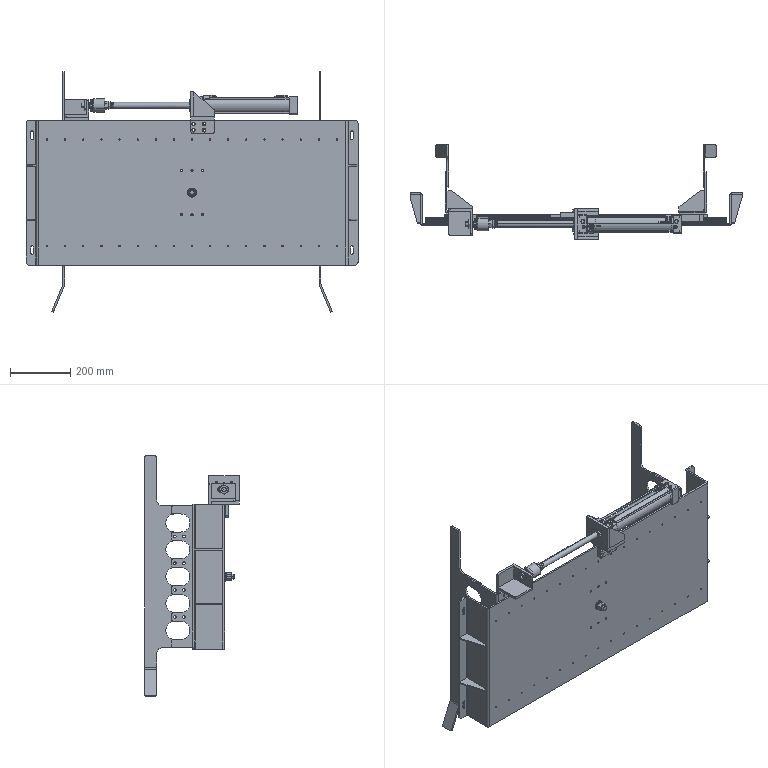Part | SolidWorks | 57 solids | 4306 faces | volume 8516253 mm3 | plane 2323 | cylinder 1338 | cone 319 | spline 240 | sphere 60 | torus 26 | commonest cylinder face diameters 1.25 x142 6 x142 9 x108 9.5 x84 10 x81 1 x80